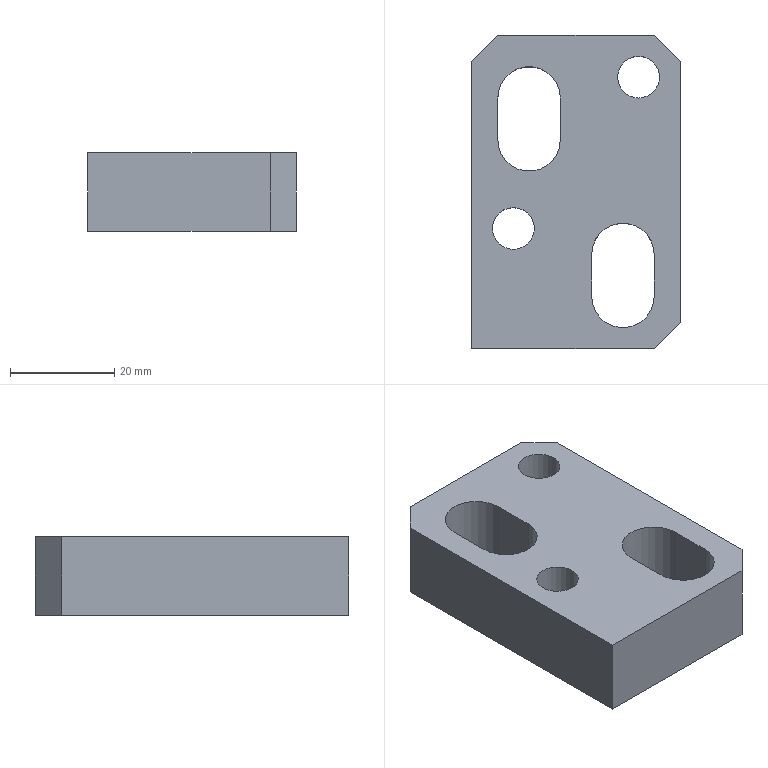Part | NX | features solid 2 | 1 solid | 19 faces | box 40 x 60 x 15 mm | volume 27657 mm3 | plane 13 | cylinder 6 | commonest cylinder face diameters 12 x4 8 x2
STEP:
#1=CARTESIAN_POINT('',(-338.,770.,-80.));
#2=VERTEX_POINT('',#1);
#3=CARTESIAN_POINT('',(-343.,765.,-80.));
#4=VERTEX_POINT('',#3);
#5=CARTESIAN_POINT('',(-338.,770.,-80.));
#6=DIRECTION('',(-0.7071,-0.7071,0.));
#7=VECTOR('',#6,1000.);
#8=LINE('',#5,#7);
#9=EDGE_CURVE('',#2,#4,#8,.T.);
#10=ORIENTED_EDGE('',*,*,#9,.T.);
#11=CARTESIAN_POINT('',(-343.,765.,-65.));
#12=VERTEX_POINT('',#11);
#13=CARTESIAN_POINT('',(-343.,765.,-65.));
#14=DIRECTION('',(0.,0.,-1.));
#15=VECTOR('',#14,1000.);
#16=LINE('',#13,#15);
#17=EDGE_CURVE('',#12,#4,#16,.T.);
#18=ORIENTED_EDGE('',*,*,#17,.F.);
#19=CARTESIAN_POINT('',(-338.,770.,-65.));
#20=VERTEX_POINT('',#19);
#21=CARTESIAN_POINT('',(-338.,770.,-65.));
#22=DIRECTION('',(-0.7071,-0.7071,0.));
#23=VECTOR('',#22,1000.);
#24=LINE('',#21,#23);
#25=EDGE_CURVE('',#20,#12,#24,.T.);
#26=ORIENTED_EDGE('',*,*,#25,.F.);
#27=CARTESIAN_POINT('',(-338.,770.,-65.));
#28=DIRECTION('',(0.,0.,-1.));
#29=VECTOR('',#28,1000.);
#30=LINE('',#27,#29);
#31=EDGE_CURVE('',#20,#2,#30,.T.);
#32=ORIENTED_EDGE('',*,*,#31,.T.);
#33=EDGE_LOOP('',(#10,#18,#26,#32));
#34=FACE_BOUND('',#33,.T.);
#35=CARTESIAN_POINT('',(-338.,770.,-65.));
#36=DIRECTION('',(-0.7071,0.7071,0.));
#37=DIRECTION('',(0.7071,0.7071,0.));
#38=AXIS2_PLACEMENT_3D('',#35,#36,#37);
#39=PLANE('',#38);
#40=ADVANCED_FACE('',(#34),#39,.T.);
#41=CARTESIAN_POINT('',(-308.,770.,-65.));
#42=VERTEX_POINT('',#41);
#43=CARTESIAN_POINT('',(-373.,770.,-65.));
#44=DIRECTION('',(1.,0.,0.));
#45=VECTOR('',#44,1000.);
#46=LINE('',#43,#45);
#47=EDGE_CURVE('',#20,#42,#46,.T.);
#48=ORIENTED_EDGE('',*,*,#47,.T.);
#49=CARTESIAN_POINT('',(-308.,770.,-80.));
#50=VERTEX_POINT('',#49);
#51=CARTESIAN_POINT('',(-308.,770.,-65.));
#52=DIRECTION('',(0.,0.,-1.));
#53=VECTOR('',#52,1000.);
#54=LINE('',#51,#53);
#55=EDGE_CURVE('',#42,#50,#54,.T.);
#56=ORIENTED_EDGE('',*,*,#55,.T.);
#57=CARTESIAN_POINT('',(-373.,770.,-80.));
#58=DIRECTION('',(1.,0.,0.));
#59=VECTOR('',#58,1000.);
#60=LINE('',#57,#59);
#61=EDGE_CURVE('',#2,#50,#60,.T.);
#62=ORIENTED_EDGE('',*,*,#61,.F.);
#63=ORIENTED_EDGE('',*,*,#31,.F.);
#64=EDGE_LOOP('',(#48,#56,#62,#63));
#65=FACE_BOUND('',#64,.T.);
#66=CARTESIAN_POINT('',(-388.,770.,-65.));
#67=DIRECTION('',(0.,1.,0.));
#68=DIRECTION('',(0.,0.,-1.));
#69=AXIS2_PLACEMENT_3D('',#66,#67,#68);
#70=PLANE('',#69);
#71=ADVANCED_FACE('',(#65),#70,.T.);
#72=CARTESIAN_POINT('',(-303.,765.,-80.));
#73=VERTEX_POINT('',#72);
#74=CARTESIAN_POINT('',(-303.,765.,-80.));
#75=DIRECTION('',(-0.7071,0.7071,0.));
#76=VECTOR('',#75,1000.);
#77=LINE('',#74,#76);
#78=EDGE_CURVE('',#73,#50,#77,.T.);
#79=ORIENTED_EDGE('',*,*,#78,.T.);
#80=ORIENTED_EDGE('',*,*,#55,.F.);
#81=CARTESIAN_POINT('',(-303.,765.,-65.));
#82=VERTEX_POINT('',#81);
#83=CARTESIAN_POINT('',(-303.,765.,-65.));
#84=DIRECTION('',(-0.7071,0.7071,0.));
#85=VECTOR('',#84,1000.);
#86=LINE('',#83,#85);
#87=EDGE_CURVE('',#82,#42,#86,.T.);
#88=ORIENTED_EDGE('',*,*,#87,.F.);
#89=CARTESIAN_POINT('',(-303.,765.,-65.));
#90=DIRECTION('',(0.,0.,-1.));
#91=VECTOR('',#90,1000.);
#92=LINE('',#89,#91);
#93=EDGE_CURVE('',#82,#73,#92,.T.);
#94=ORIENTED_EDGE('',*,*,#93,.T.);
#95=EDGE_LOOP('',(#79,#80,#88,#94));
#96=FACE_BOUND('',#95,.T.);
#97=CARTESIAN_POINT('',(-303.,765.,-65.));
#98=DIRECTION('',(0.7071,0.7071,0.));
#99=DIRECTION('',(0.7071,-0.7071,0.));
#100=AXIS2_PLACEMENT_3D('',#97,#98,#99);
#101=PLANE('',#100);
#102=ADVANCED_FACE('',(#96),#101,.T.);
#103=CARTESIAN_POINT('',(-303.,715.,-80.));
#104=VERTEX_POINT('',#103);
#105=CARTESIAN_POINT('',(-303.,735.,-80.));
#106=DIRECTION('',(0.,1.,0.));
#107=VECTOR('',#106,1000.);
#108=LINE('',#105,#107);
#109=EDGE_CURVE('',#104,#73,#108,.T.);
#110=ORIENTED_EDGE('',*,*,#109,.T.);
#111=ORIENTED_EDGE('',*,*,#93,.F.);
#112=CARTESIAN_POINT('',(-303.,715.,-65.));
#113=VERTEX_POINT('',#112);
#114=CARTESIAN_POINT('',(-303.,735.,-65.));
#115=DIRECTION('',(0.,1.,0.));
#116=VECTOR('',#115,1000.);
#117=LINE('',#114,#116);
#118=EDGE_CURVE('',#113,#82,#117,.T.);
#119=ORIENTED_EDGE('',*,*,#118,.F.);
#120=CARTESIAN_POINT('',(-303.,715.,-65.));
#121=DIRECTION('',(0.,0.,-1.));
#122=VECTOR('',#121,1000.);
#123=LINE('',#120,#122);
#124=EDGE_CURVE('',#113,#104,#123,.T.);
#125=ORIENTED_EDGE('',*,*,#124,.T.);
#126=EDGE_LOOP('',(#110,#111,#119,#125));
#127=FACE_BOUND('',#126,.T.);
#128=CARTESIAN_POINT('',(-303.,735.,-65.));
#129=DIRECTION('',(1.,0.,0.));
#130=DIRECTION('',(0.,-1.,0.));
#131=AXIS2_PLACEMENT_3D('',#128,#129,#130);
#132=PLANE('',#131);
#133=ADVANCED_FACE('',(#127),#132,.T.);
#134=CARTESIAN_POINT('',(-308.,710.,-80.));
#135=VERTEX_POINT('',#134);
#136=CARTESIAN_POINT('',(-308.,710.,-80.));
#137=DIRECTION('',(0.7071,0.7071,0.));
#138=VECTOR('',#137,1000.);
#139=LINE('',#136,#138);
#140=EDGE_CURVE('',#135,#104,#139,.T.);
#141=ORIENTED_EDGE('',*,*,#140,.T.);
#142=ORIENTED_EDGE('',*,*,#124,.F.);
#143=CARTESIAN_POINT('',(-308.,710.,-65.));
#144=VERTEX_POINT('',#143);
#145=CARTESIAN_POINT('',(-308.,710.,-65.));
#146=DIRECTION('',(0.7071,0.7071,0.));
#147=VECTOR('',#146,1000.);
#148=LINE('',#145,#147);
#149=EDGE_CURVE('',#144,#113,#148,.T.);
#150=ORIENTED_EDGE('',*,*,#149,.F.);
#151=CARTESIAN_POINT('',(-308.,710.,-65.));
#152=DIRECTION('',(0.,0.,-1.));
#153=VECTOR('',#152,1000.);
#154=LINE('',#151,#153);
#155=EDGE_CURVE('',#144,#135,#154,.T.);
#156=ORIENTED_EDGE('',*,*,#155,.T.);
#157=EDGE_LOOP('',(#141,#142,#150,#156));
#158=FACE_BOUND('',#157,.T.);
#159=CARTESIAN_POINT('',(-308.,710.,-65.));
#160=DIRECTION('',(0.7071,-0.7071,0.));
#161=DIRECTION('',(-0.7071,-0.7071,0.));
#162=AXIS2_PLACEMENT_3D('',#159,#160,#161);
#163=PLANE('',#162);
#164=ADVANCED_FACE('',(#158),#163,.T.);
#165=CARTESIAN_POINT('',(-326.,750.,-65.));
#166=VERTEX_POINT('',#165);
#167=CARTESIAN_POINT('',(-338.,750.,-65.));
#168=VERTEX_POINT('',#167);
#169=CARTESIAN_POINT('',(-332.,750.,-65.));
#170=DIRECTION('',(0.,0.,-1.));
#171=DIRECTION('',(0.,1.,0.));
#172=AXIS2_PLACEMENT_3D('',#169,#170,#171);
#173=CIRCLE('',#172,6.);
#174=EDGE_CURVE('',#166,#168,#173,.T.);
#175=ORIENTED_EDGE('',*,*,#174,.F.);
#176=CARTESIAN_POINT('',(-326.,750.,-80.));
#177=VERTEX_POINT('',#176);
#178=CARTESIAN_POINT('',(-326.,750.,-65.));
#179=DIRECTION('',(0.,0.,-1.));
#180=VECTOR('',#179,1000.);
#181=LINE('',#178,#180);
#182=EDGE_CURVE('',#166,#177,#181,.T.);
#183=ORIENTED_EDGE('',*,*,#182,.T.);
#184=CARTESIAN_POINT('',(-338.,750.,-80.));
#185=VERTEX_POINT('',#184);
#186=CARTESIAN_POINT('',(-332.,750.,-80.));
#187=DIRECTION('',(0.,0.,-1.));
#188=DIRECTION('',(0.,1.,0.));
#189=AXIS2_PLACEMENT_3D('',#186,#187,#188);
#190=CIRCLE('',#189,6.);
#191=EDGE_CURVE('',#177,#185,#190,.T.);
#192=ORIENTED_EDGE('',*,*,#191,.T.);
#193=CARTESIAN_POINT('',(-338.,750.,-65.));
#194=DIRECTION('',(0.,0.,-1.));
#195=VECTOR('',#194,1000.);
#196=LINE('',#193,#195);
#197=EDGE_CURVE('',#168,#185,#196,.T.);
#198=ORIENTED_EDGE('',*,*,#197,.F.);
#199=EDGE_LOOP('',(#175,#183,#192,#198));
#200=FACE_BOUND('',#199,.T.);
#201=CARTESIAN_POINT('',(-332.,750.,-65.));
#202=DIRECTION('',(0.,0.,-1.));
#203=DIRECTION('',(0.,-1.,0.));
#204=AXIS2_PLACEMENT_3D('',#201,#202,#203);
#205=CYLINDRICAL_SURFACE('',#204,6.);
#206=ADVANCED_FACE('',(#200),#205,.F.);
#207=CARTESIAN_POINT('',(-326.,758.,-80.));
#208=VERTEX_POINT('',#207);
#209=CARTESIAN_POINT('',(-326.,725.,-80.));
#210=DIRECTION('',(0.,1.,0.));
#211=VECTOR('',#210,1000.);
#212=LINE('',#209,#211);
#213=EDGE_CURVE('',#177,#208,#212,.T.);
#214=ORIENTED_EDGE('',*,*,#213,.F.);
#215=ORIENTED_EDGE('',*,*,#182,.F.);
#216=CARTESIAN_POINT('',(-326.,758.,-65.));
#217=VERTEX_POINT('',#216);
#218=CARTESIAN_POINT('',(-326.,725.,-65.));
#219=DIRECTION('',(0.,1.,0.));
#220=VECTOR('',#219,1000.);
#221=LINE('',#218,#220);
#222=EDGE_CURVE('',#166,#217,#221,.T.);
#223=ORIENTED_EDGE('',*,*,#222,.T.);
#224=CARTESIAN_POINT('',(-326.,758.,-65.));
#225=DIRECTION('',(0.,0.,-1.));
#226=VECTOR('',#225,1000.);
#227=LINE('',#224,#226);
#228=EDGE_CURVE('',#217,#208,#227,.T.);
#229=ORIENTED_EDGE('',*,*,#228,.T.);
#230=EDGE_LOOP('',(#214,#215,#223,#229));
#231=FACE_BOUND('',#230,.T.);
#232=CARTESIAN_POINT('',(-326.,725.,-65.));
#233=DIRECTION('',(1.,0.,0.));
#234=DIRECTION('',(0.,-1.,0.));
#235=AXIS2_PLACEMENT_3D('',#232,#233,#234);
#236=PLANE('',#235);
#237=ADVANCED_FACE('',(#231),#236,.F.);
#238=CARTESIAN_POINT('',(-338.,758.,-80.));
#239=VERTEX_POINT('',#238);
#240=CARTESIAN_POINT('',(-332.,758.,-80.));
#241=DIRECTION('',(0.,0.,-1.));
#242=DIRECTION('',(0.,1.,0.));
#243=AXIS2_PLACEMENT_3D('',#240,#241,#242);
#244=CIRCLE('',#243,6.);
#245=EDGE_CURVE('',#239,#208,#244,.T.);
#246=ORIENTED_EDGE('',*,*,#245,.T.);
#247=ORIENTED_EDGE('',*,*,#228,.F.);
#248=CARTESIAN_POINT('',(-338.,758.,-65.));
#249=VERTEX_POINT('',#248);
#250=CARTESIAN_POINT('',(-332.,758.,-65.));
#251=DIRECTION('',(0.,0.,-1.));
#252=DIRECTION('',(0.,1.,0.));
#253=AXIS2_PLACEMENT_3D('',#250,#251,#252);
#254=CIRCLE('',#253,6.);
#255=EDGE_CURVE('',#249,#217,#254,.T.);
#256=ORIENTED_EDGE('',*,*,#255,.F.);
#257=CARTESIAN_POINT('',(-338.,758.,-65.));
#258=DIRECTION('',(0.,0.,-1.));
#259=VECTOR('',#258,1000.);
#260=LINE('',#257,#259);
#261=EDGE_CURVE('',#249,#239,#260,.T.);
#262=ORIENTED_EDGE('',*,*,#261,.T.);
#263=EDGE_LOOP('',(#246,#247,#256,#262));
#264=FACE_BOUND('',#263,.T.);
#265=CARTESIAN_POINT('',(-332.,758.,-65.));
#266=DIRECTION('',(0.,0.,-1.));
#267=DIRECTION('',(0.,-1.,0.));
#268=AXIS2_PLACEMENT_3D('',#265,#266,#267);
#269=CYLINDRICAL_SURFACE('',#268,6.);
#270=ADVANCED_FACE('',(#264),#269,.F.);
#271=CARTESIAN_POINT('',(-338.,733.,-80.));
#272=DIRECTION('',(0.,-1.,0.));
#273=VECTOR('',#272,1000.);
#274=LINE('',#271,#273);
#275=EDGE_CURVE('',#239,#185,#274,.T.);
#276=ORIENTED_EDGE('',*,*,#275,.F.);
#277=ORIENTED_EDGE('',*,*,#261,.F.);
#278=CARTESIAN_POINT('',(-338.,733.,-65.));
#279=DIRECTION('',(0.,-1.,0.));
#280=VECTOR('',#279,1000.);
#281=LINE('',#278,#280);
#282=EDGE_CURVE('',#249,#168,#281,.T.);
#283=ORIENTED_EDGE('',*,*,#282,.T.);
#284=ORIENTED_EDGE('',*,*,#197,.T.);
#285=EDGE_LOOP('',(#276,#277,#283,#284));
#286=FACE_BOUND('',#285,.T.);
#287=CARTESIAN_POINT('',(-338.,733.,-65.));
#288=DIRECTION('',(-1.,0.,0.));
#289=DIRECTION('',(0.,0.,-1.));
#290=AXIS2_PLACEMENT_3D('',#287,#288,#289);
#291=PLANE('',#290);
#292=ADVANCED_FACE('',(#286),#291,.F.);
#293=CARTESIAN_POINT('',(-311.,766.,-65.));
#294=VERTEX_POINT('',#293);
#295=CARTESIAN_POINT('',(-311.,762.,-65.));
#296=DIRECTION('',(0.,0.,-1.));
#297=DIRECTION('',(0.,1.,0.));
#298=AXIS2_PLACEMENT_3D('',#295,#296,#297);
#299=CIRCLE('',#298,4.);
#300=EDGE_CURVE('',#294,#294,#299,.T.);
#301=ORIENTED_EDGE('',*,*,#300,.F.);
#302=EDGE_LOOP('',(#301));
#303=FACE_BOUND('',#302,.T.);
#304=CARTESIAN_POINT('',(-311.,766.,-80.));
#305=VERTEX_POINT('',#304);
#306=CARTESIAN_POINT('',(-311.,762.,-80.));
#307=DIRECTION('',(0.,0.,-1.));
#308=DIRECTION('',(0.,1.,0.));
#309=AXIS2_PLACEMENT_3D('',#306,#307,#308);
#310=CIRCLE('',#309,4.);
#311=EDGE_CURVE('',#305,#305,#310,.T.);
#312=ORIENTED_EDGE('',*,*,#311,.T.);
#313=EDGE_LOOP('',(#312));
#314=FACE_BOUND('',#313,.T.);
#315=CARTESIAN_POINT('',(-311.,762.,-65.));
#316=DIRECTION('',(0.,0.,-1.));
#317=DIRECTION('',(0.,-1.,0.));
#318=AXIS2_PLACEMENT_3D('',#315,#316,#317);
#319=CYLINDRICAL_SURFACE('',#318,4.);
#320=ADVANCED_FACE('',(#303,#314),#319,.F.);
#321=CARTESIAN_POINT('',(-308.,720.,-80.));
#322=VERTEX_POINT('',#321);
#323=CARTESIAN_POINT('',(-320.,720.,-80.));
#324=VERTEX_POINT('',#323);
#325=CARTESIAN_POINT('',(-314.,720.,-80.));
#326=DIRECTION('',(0.,0.,-1.));
#327=DIRECTION('',(0.,1.,0.));
#328=AXIS2_PLACEMENT_3D('',#325,#326,#327);
#329=CIRCLE('',#328,6.);
#330=EDGE_CURVE('',#322,#324,#329,.T.);
#331=ORIENTED_EDGE('',*,*,#330,.T.);
#332=CARTESIAN_POINT('',(-320.,720.,-65.));
#333=VERTEX_POINT('',#332);
#334=CARTESIAN_POINT('',(-320.,720.,-65.));
#335=DIRECTION('',(0.,0.,-1.));
#336=VECTOR('',#335,1000.);
#337=LINE('',#334,#336);
#338=EDGE_CURVE('',#333,#324,#337,.T.);
#339=ORIENTED_EDGE('',*,*,#338,.F.);
#340=CARTESIAN_POINT('',(-308.,720.,-65.));
#341=VERTEX_POINT('',#340);
#342=CARTESIAN_POINT('',(-314.,720.,-65.));
#343=DIRECTION('',(0.,0.,-1.));
#344=DIRECTION('',(0.,1.,0.));
#345=AXIS2_PLACEMENT_3D('',#342,#343,#344);
#346=CIRCLE('',#345,6.);
#347=EDGE_CURVE('',#341,#333,#346,.T.);
#348=ORIENTED_EDGE('',*,*,#347,.F.);
#349=CARTESIAN_POINT('',(-308.,720.,-65.));
#350=DIRECTION('',(0.,0.,-1.));
#351=VECTOR('',#350,1000.);
#352=LINE('',#349,#351);
#353=EDGE_CURVE('',#341,#322,#352,.T.);
#354=ORIENTED_EDGE('',*,*,#353,.T.);
#355=EDGE_LOOP('',(#331,#339,#348,#354));
#356=FACE_BOUND('',#355,.T.);
#357=CARTESIAN_POINT('',(-314.,720.,-65.));
#358=DIRECTION('',(0.,0.,-1.));
#359=DIRECTION('',(0.,-1.,0.));
#360=AXIS2_PLACEMENT_3D('',#357,#358,#359);
#361=CYLINDRICAL_SURFACE('',#360,6.);
#362=ADVANCED_FACE('',(#356),#361,.F.);
#363=CARTESIAN_POINT('',(-308.,728.,-80.));
#364=VERTEX_POINT('',#363);
#365=CARTESIAN_POINT('',(-308.,715.,-80.));
#366=DIRECTION('',(0.,1.,0.));
#367=VECTOR('',#366,1000.);
#368=LINE('',#365,#367);
#369=EDGE_CURVE('',#322,#364,#368,.T.);
#370=ORIENTED_EDGE('',*,*,#369,.F.);
#371=ORIENTED_EDGE('',*,*,#353,.F.);
#372=CARTESIAN_POINT('',(-308.,728.,-65.));
#373=VERTEX_POINT('',#372);
#374=CARTESIAN_POINT('',(-308.,715.,-65.));
#375=DIRECTION('',(0.,1.,0.));
#376=VECTOR('',#375,1000.);
#377=LINE('',#374,#376);
#378=EDGE_CURVE('',#341,#373,#377,.T.);
#379=ORIENTED_EDGE('',*,*,#378,.T.);
#380=CARTESIAN_POINT('',(-308.,728.,-65.));
#381=DIRECTION('',(0.,0.,-1.));
#382=VECTOR('',#381,1000.);
#383=LINE('',#380,#382);
#384=EDGE_CURVE('',#373,#364,#383,.T.);
#385=ORIENTED_EDGE('',*,*,#384,.T.);
#386=EDGE_LOOP('',(#370,#371,#379,#385));
#387=FACE_BOUND('',#386,.T.);
#388=CARTESIAN_POINT('',(-308.,715.,-65.));
#389=DIRECTION('',(1.,0.,0.));
#390=DIRECTION('',(0.,0.,1.));
#391=AXIS2_PLACEMENT_3D('',#388,#389,#390);
#392=PLANE('',#391);
#393=ADVANCED_FACE('',(#387),#392,.F.);
#394=CARTESIAN_POINT('',(-320.,728.,-80.));
#395=VERTEX_POINT('',#394);
#396=CARTESIAN_POINT('',(-314.,728.,-80.));
#397=DIRECTION('',(0.,0.,-1.));
#398=DIRECTION('',(0.,1.,0.));
#399=AXIS2_PLACEMENT_3D('',#396,#397,#398);
#400=CIRCLE('',#399,6.);
#401=EDGE_CURVE('',#395,#364,#400,.T.);
#402=ORIENTED_EDGE('',*,*,#401,.T.);
#403=ORIENTED_EDGE('',*,*,#384,.F.);
#404=CARTESIAN_POINT('',(-320.,728.,-65.));
#405=VERTEX_POINT('',#404);
#406=CARTESIAN_POINT('',(-314.,728.,-65.));
#407=DIRECTION('',(0.,0.,-1.));
#408=DIRECTION('',(0.,1.,0.));
#409=AXIS2_PLACEMENT_3D('',#406,#407,#408);
#410=CIRCLE('',#409,6.);
#411=EDGE_CURVE('',#405,#373,#410,.T.);
#412=ORIENTED_EDGE('',*,*,#411,.F.);
#413=CARTESIAN_POINT('',(-320.,728.,-65.));
#414=DIRECTION('',(0.,0.,-1.));
#415=VECTOR('',#414,1000.);
#416=LINE('',#413,#415);
#417=EDGE_CURVE('',#405,#395,#416,.T.);
#418=ORIENTED_EDGE('',*,*,#417,.T.);
#419=EDGE_LOOP('',(#402,#403,#412,#418));
#420=FACE_BOUND('',#419,.T.);
#421=CARTESIAN_POINT('',(-314.,728.,-65.));
#422=DIRECTION('',(0.,0.,-1.));
#423=DIRECTION('',(0.,-1.,0.));
#424=AXIS2_PLACEMENT_3D('',#421,#422,#423);
#425=CYLINDRICAL_SURFACE('',#424,6.);
#426=ADVANCED_FACE('',(#420),#425,.F.);
#427=CARTESIAN_POINT('',(-320.,723.,-80.));
#428=DIRECTION('',(0.,-1.,0.));
#429=VECTOR('',#428,1000.);
#430=LINE('',#427,#429);
#431=EDGE_CURVE('',#395,#324,#430,.T.);
#432=ORIENTED_EDGE('',*,*,#431,.F.);
#433=ORIENTED_EDGE('',*,*,#417,.F.);
#434=CARTESIAN_POINT('',(-320.,723.,-65.));
#435=DIRECTION('',(0.,-1.,0.));
#436=VECTOR('',#435,1000.);
#437=LINE('',#434,#436);
#438=EDGE_CURVE('',#405,#333,#437,.T.);
#439=ORIENTED_EDGE('',*,*,#438,.T.);
#440=ORIENTED_EDGE('',*,*,#338,.T.);
#441=EDGE_LOOP('',(#432,#433,#439,#440));
#442=FACE_BOUND('',#441,.T.);
#443=CARTESIAN_POINT('',(-320.,723.,-65.));
#444=DIRECTION('',(-1.,0.,0.));
#445=DIRECTION('',(0.,1.,0.));
#446=AXIS2_PLACEMENT_3D('',#443,#444,#445);
#447=PLANE('',#446);
#448=ADVANCED_FACE('',(#442),#447,.F.);
#449=CARTESIAN_POINT('',(-335.,737.,-65.));
#450=VERTEX_POINT('',#449);
#451=CARTESIAN_POINT('',(-335.,733.,-65.));
#452=DIRECTION('',(0.,0.,-1.));
#453=DIRECTION('',(0.,1.,0.));
#454=AXIS2_PLACEMENT_3D('',#451,#452,#453);
#455=CIRCLE('',#454,4.);
#456=EDGE_CURVE('',#450,#450,#455,.T.);
#457=ORIENTED_EDGE('',*,*,#456,.F.);
#458=EDGE_LOOP('',(#457));
#459=FACE_BOUND('',#458,.T.);
#460=CARTESIAN_POINT('',(-335.,737.,-80.));
#461=VERTEX_POINT('',#460);
#462=CARTESIAN_POINT('',(-335.,733.,-80.));
#463=DIRECTION('',(0.,0.,-1.));
#464=DIRECTION('',(0.,1.,0.));
#465=AXIS2_PLACEMENT_3D('',#462,#463,#464);
#466=CIRCLE('',#465,4.);
#467=EDGE_CURVE('',#461,#461,#466,.T.);
#468=ORIENTED_EDGE('',*,*,#467,.T.);
#469=EDGE_LOOP('',(#468));
#470=FACE_BOUND('',#469,.T.);
#471=CARTESIAN_POINT('',(-335.,733.,-65.));
#472=DIRECTION('',(0.,0.,-1.));
#473=DIRECTION('',(0.,-1.,0.));
#474=AXIS2_PLACEMENT_3D('',#471,#472,#473);
#475=CYLINDRICAL_SURFACE('',#474,4.);
#476=ADVANCED_FACE('',(#459,#470),#475,.F.);
#477=CARTESIAN_POINT('',(-343.,710.,-65.));
#478=VERTEX_POINT('',#477);
#479=CARTESIAN_POINT('',(-343.,765.,-65.));
#480=DIRECTION('',(0.,-1.,0.));
#481=VECTOR('',#480,1000.);
#482=LINE('',#479,#481);
#483=EDGE_CURVE('',#12,#478,#482,.T.);
#484=ORIENTED_EDGE('',*,*,#483,.F.);
#485=ORIENTED_EDGE('',*,*,#17,.T.);
#486=CARTESIAN_POINT('',(-343.,710.,-80.));
#487=VERTEX_POINT('',#486);
#488=CARTESIAN_POINT('',(-343.,835.,-80.));
#489=DIRECTION('',(0.,1.,0.));
#490=VECTOR('',#489,1000.);
#491=LINE('',#488,#490);
#492=EDGE_CURVE('',#487,#4,#491,.T.);
#493=ORIENTED_EDGE('',*,*,#492,.F.);
#494=CARTESIAN_POINT('',(-343.,710.,-65.));
#495=DIRECTION('',(0.,0.,1.));
#496=VECTOR('',#495,1000.);
#497=LINE('',#494,#496);
#498=EDGE_CURVE('',#478,#487,#497,.F.);
#499=ORIENTED_EDGE('',*,*,#498,.F.);
#500=EDGE_LOOP('',(#484,#485,#493,#499));
#501=FACE_BOUND('',#500,.T.);
#502=CARTESIAN_POINT('',(-343.,737.,-65.));
#503=DIRECTION('',(-1.,0.,0.));
#504=DIRECTION('',(0.,0.,-1.));
#505=AXIS2_PLACEMENT_3D('',#502,#503,#504);
#506=PLANE('',#505);
#507=ADVANCED_FACE('',(#501),#506,.T.);
#508=CARTESIAN_POINT('',(-388.,710.,-65.));
#509=DIRECTION('',(1.,0.,0.));
#510=VECTOR('',#509,1000.);
#511=LINE('',#508,#510);
#512=EDGE_CURVE('',#478,#144,#511,.T.);
#513=ORIENTED_EDGE('',*,*,#512,.F.);
#514=ORIENTED_EDGE('',*,*,#498,.T.);
#515=CARTESIAN_POINT('',(-346.,710.,-80.));
#516=DIRECTION('',(-1.,0.,0.));
#517=VECTOR('',#516,1000.);
#518=LINE('',#515,#517);
#519=EDGE_CURVE('',#487,#135,#518,.F.);
#520=ORIENTED_EDGE('',*,*,#519,.T.);
#521=ORIENTED_EDGE('',*,*,#155,.F.);
#522=EDGE_LOOP('',(#513,#514,#520,#521));
#523=FACE_BOUND('',#522,.T.);
#524=CARTESIAN_POINT('',(-388.,710.,-65.));
#525=DIRECTION('',(0.,-1.,0.));
#526=DIRECTION('',(-1.,0.,0.));
#527=AXIS2_PLACEMENT_3D('',#524,#525,#526);
#528=PLANE('',#527);
#529=ADVANCED_FACE('',(#523),#528,.T.);
#530=ORIENTED_EDGE('',*,*,#467,.F.);
#531=EDGE_LOOP('',(#530));
#532=FACE_BOUND('',#531,.T.);
#533=ORIENTED_EDGE('',*,*,#431,.T.);
#534=ORIENTED_EDGE('',*,*,#330,.F.);
#535=ORIENTED_EDGE('',*,*,#369,.T.);
#536=ORIENTED_EDGE('',*,*,#401,.F.);
#537=EDGE_LOOP('',(#533,#534,#535,#536));
#538=FACE_BOUND('',#537,.T.);
#539=ORIENTED_EDGE('',*,*,#311,.F.);
#540=EDGE_LOOP('',(#539));
#541=FACE_BOUND('',#540,.T.);
#542=ORIENTED_EDGE('',*,*,#275,.T.);
#543=ORIENTED_EDGE('',*,*,#191,.F.);
#544=ORIENTED_EDGE('',*,*,#213,.T.);
#545=ORIENTED_EDGE('',*,*,#245,.F.);
#546=EDGE_LOOP('',(#542,#543,#544,#545));
#547=FACE_BOUND('',#546,.T.);
#548=ORIENTED_EDGE('',*,*,#519,.F.);
#549=ORIENTED_EDGE('',*,*,#492,.T.);
#550=ORIENTED_EDGE('',*,*,#9,.F.);
#551=ORIENTED_EDGE('',*,*,#61,.T.);
#552=ORIENTED_EDGE('',*,*,#78,.F.);
#553=ORIENTED_EDGE('',*,*,#109,.F.);
#554=ORIENTED_EDGE('',*,*,#140,.F.);
#555=EDGE_LOOP('',(#548,#549,#550,#551,#552,#553,#554));
#556=FACE_BOUND('',#555,.T.);
#557=CARTESIAN_POINT('',(-346.,835.,-80.));
#558=DIRECTION('',(0.,0.,1.));
#559=DIRECTION('',(-1.,0.,0.));
#560=AXIS2_PLACEMENT_3D('',#557,#558,#559);
#561=PLANE('',#560);
#562=ADVANCED_FACE('',(#532,#538,#541,#547,#556),#561,.F.);
#563=ORIENTED_EDGE('',*,*,#149,.T.);
#564=ORIENTED_EDGE('',*,*,#118,.T.);
#565=ORIENTED_EDGE('',*,*,#87,.T.);
#566=ORIENTED_EDGE('',*,*,#47,.F.);
#567=ORIENTED_EDGE('',*,*,#25,.T.);
#568=ORIENTED_EDGE('',*,*,#483,.T.);
#569=ORIENTED_EDGE('',*,*,#512,.T.);
#570=EDGE_LOOP('',(#563,#564,#565,#566,#567,#568,#569));
#571=FACE_BOUND('',#570,.T.);
#572=ORIENTED_EDGE('',*,*,#456,.T.);
#573=EDGE_LOOP('',(#572));
#574=FACE_BOUND('',#573,.T.);
#575=ORIENTED_EDGE('',*,*,#300,.T.);
#576=EDGE_LOOP('',(#575));
#577=FACE_BOUND('',#576,.T.);
#578=ORIENTED_EDGE('',*,*,#438,.F.);
#579=ORIENTED_EDGE('',*,*,#411,.T.);
#580=ORIENTED_EDGE('',*,*,#378,.F.);
#581=ORIENTED_EDGE('',*,*,#347,.T.);
#582=EDGE_LOOP('',(#578,#579,#580,#581));
#583=FACE_BOUND('',#582,.T.);
#584=ORIENTED_EDGE('',*,*,#255,.T.);
#585=ORIENTED_EDGE('',*,*,#222,.F.);
#586=ORIENTED_EDGE('',*,*,#174,.T.);
#587=ORIENTED_EDGE('',*,*,#282,.F.);
#588=EDGE_LOOP('',(#584,#585,#586,#587));
#589=FACE_BOUND('',#588,.T.);
#590=CARTESIAN_POINT('',(-346.,835.,-65.));
#591=DIRECTION('',(0.,0.,1.));
#592=DIRECTION('',(-1.,0.,0.));
#593=AXIS2_PLACEMENT_3D('',#590,#591,#592);
#594=PLANE('',#593);
#595=ADVANCED_FACE('',(#571,#574,#577,#583,#589),#594,.T.);
#596=CLOSED_SHELL('',(#40,#71,#102,#133,#164,#206,#237,#270,#292,#320,#362,#393,#426,#448,#476,#507,#529,#562,#595));
#597=MANIFOLD_SOLID_BREP('',#596);
#598=(LENGTH_UNIT()NAMED_UNIT(*)SI_UNIT(.MILLI.,.METRE.));
#599=UNCERTAINTY_MEASURE_WITH_UNIT(LENGTH_MEASURE(0.00001),#598,'','');
#600=(NAMED_UNIT(*)PLANE_ANGLE_UNIT()SI_UNIT($,.RADIAN.));
#601=(NAMED_UNIT(*)SI_UNIT($,.STERADIAN.)SOLID_ANGLE_UNIT());
#602=(GEOMETRIC_REPRESENTATION_CONTEXT(3)GLOBAL_UNCERTAINTY_ASSIGNED_CONTEXT((#599))GLOBAL_UNIT_ASSIGNED_CONTEXT((#598,#600,#601))REPRESENTATION_CONTEXT('',''));
#603=ADVANCED_BREP_SHAPE_REPRESENTATION('',(#597),#602);